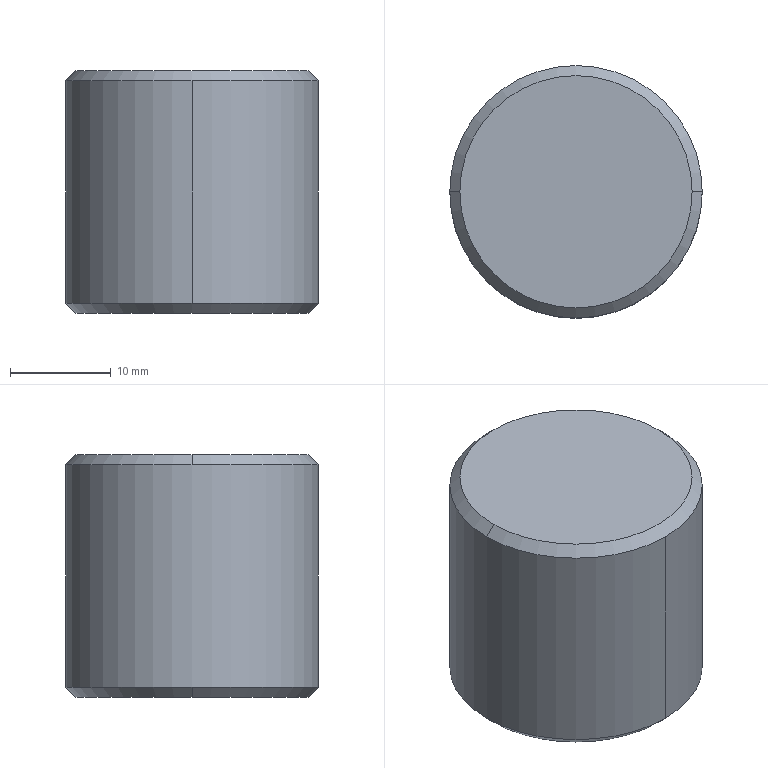Part | Creo | 1 solid | 8 faces | box 25 x 25 x 24 mm | volume 11705 mm3 | cone 4 | plane 2 | cylinder 2 | commonest cylinder face diameters 25 x2
STEP:
#1=CARTESIAN_POINT('',(-132.,-250.505,-316.));
#2=VERTEX_POINT('',#1);
#3=CARTESIAN_POINT('',(-120.5,-262.005,-316.));
#4=VERTEX_POINT('',#3);
#5=CARTESIAN_POINT('',(-132.,-262.005,-316.));
#6=DIRECTION('',(0.,0.,-1.));
#7=DIRECTION('',(0.,1.,0.));
#8=AXIS2_PLACEMENT_3D('',#5,#6,#7);
#9=CIRCLE('',#8,11.5);
#10=EDGE_CURVE('',#2,#4,#9,.T.);
#11=ORIENTED_EDGE('',*,*,#10,.F.);
#12=CARTESIAN_POINT('',(-143.5,-262.005,-316.));
#13=VERTEX_POINT('',#12);
#14=CARTESIAN_POINT('',(-132.,-262.005,-316.));
#15=DIRECTION('',(0.,0.,-1.));
#16=DIRECTION('',(-1.,0.,0.));
#17=AXIS2_PLACEMENT_3D('',#14,#15,#16);
#18=CIRCLE('',#17,11.5);
#19=EDGE_CURVE('',#13,#2,#18,.T.);
#20=ORIENTED_EDGE('',*,*,#19,.F.);
#21=CARTESIAN_POINT('',(-132.,-273.505,-316.));
#22=VERTEX_POINT('',#21);
#23=CARTESIAN_POINT('',(-132.,-262.005,-316.));
#24=DIRECTION('',(0.,0.,-1.));
#25=DIRECTION('',(0.,-1.,0.));
#26=AXIS2_PLACEMENT_3D('',#23,#24,#25);
#27=CIRCLE('',#26,11.5);
#28=EDGE_CURVE('',#22,#13,#27,.T.);
#29=ORIENTED_EDGE('',*,*,#28,.F.);
#30=CARTESIAN_POINT('',(-132.,-262.005,-316.));
#31=DIRECTION('',(0.,0.,-1.));
#32=DIRECTION('',(1.,0.,0.));
#33=AXIS2_PLACEMENT_3D('',#30,#31,#32);
#34=CIRCLE('',#33,11.5);
#35=EDGE_CURVE('',#4,#22,#34,.T.);
#36=ORIENTED_EDGE('',*,*,#35,.F.);
#37=EDGE_LOOP('',(#11,#20,#29,#36));
#38=FACE_OUTER_BOUND('',#37,.F.);
#39=CARTESIAN_POINT('',(-10.,7.995,-316.));
#40=DIRECTION('',(0.,0.,1.));
#41=DIRECTION('',(0.,-1.,0.));
#42=AXIS2_PLACEMENT_3D('',#39,#40,#41);
#43=PLANE('',#42);
#44=ADVANCED_FACE('',(#38),#43,.F.);
#45=ORIENTED_EDGE('',*,*,#19,.T.);
#46=ORIENTED_EDGE('',*,*,#10,.T.);
#47=CARTESIAN_POINT('',(-119.5,-262.005,-315.));
#48=VERTEX_POINT('',#47);
#49=CARTESIAN_POINT('',(-120.5,-262.005,-316.));
#50=DIRECTION('',(0.7071,0.,0.7071));
#51=VECTOR('',#50,1.414);
#52=LINE('',#49,#51);
#53=EDGE_CURVE('',#4,#48,#52,.T.);
#54=ORIENTED_EDGE('',*,*,#53,.T.);
#55=CARTESIAN_POINT('',(-132.,-249.505,-315.));
#56=VERTEX_POINT('',#55);
#57=CARTESIAN_POINT('',(-132.,-262.005,-315.));
#58=DIRECTION('',(0.,0.,-1.));
#59=DIRECTION('',(0.,1.,0.));
#60=AXIS2_PLACEMENT_3D('',#57,#58,#59);
#61=CIRCLE('',#60,12.5);
#62=EDGE_CURVE('',#56,#48,#61,.T.);
#63=ORIENTED_EDGE('',*,*,#62,.F.);
#64=CARTESIAN_POINT('',(-144.5,-262.005,-315.));
#65=VERTEX_POINT('',#64);
#66=CARTESIAN_POINT('',(-132.,-262.005,-315.));
#67=DIRECTION('',(0.,0.,-1.));
#68=DIRECTION('',(-1.,0.,0.));
#69=AXIS2_PLACEMENT_3D('',#66,#67,#68);
#70=CIRCLE('',#69,12.5);
#71=EDGE_CURVE('',#65,#56,#70,.T.);
#72=ORIENTED_EDGE('',*,*,#71,.F.);
#73=CARTESIAN_POINT('',(-143.5,-262.005,-316.));
#74=DIRECTION('',(-0.7071,0.,0.7071));
#75=VECTOR('',#74,1.414);
#76=LINE('',#73,#75);
#77=EDGE_CURVE('',#13,#65,#76,.T.);
#78=ORIENTED_EDGE('',*,*,#77,.F.);
#79=EDGE_LOOP('',(#45,#46,#54,#63,#72,#78));
#80=FACE_OUTER_BOUND('',#79,.F.);
#81=CARTESIAN_POINT('',(-132.,-262.005,-315.5));
#82=DIRECTION('',(0.,0.,1.));
#83=DIRECTION('',(-1.,0.,0.));
#84=AXIS2_PLACEMENT_3D('',#81,#82,#83);
#85=CONICAL_SURFACE('',#84,12.,45.);
#86=ADVANCED_FACE('',(#80),#85,.T.);
#87=ORIENTED_EDGE('',*,*,#28,.T.);
#88=ORIENTED_EDGE('',*,*,#77,.T.);
#89=CARTESIAN_POINT('',(-132.,-274.505,-315.));
#90=VERTEX_POINT('',#89);
#91=CARTESIAN_POINT('',(-132.,-262.005,-315.));
#92=DIRECTION('',(0.,0.,-1.));
#93=DIRECTION('',(0.,-1.,0.));
#94=AXIS2_PLACEMENT_3D('',#91,#92,#93);
#95=CIRCLE('',#94,12.5);
#96=EDGE_CURVE('',#90,#65,#95,.T.);
#97=ORIENTED_EDGE('',*,*,#96,.F.);
#98=CARTESIAN_POINT('',(-132.,-262.005,-315.));
#99=DIRECTION('',(0.,0.,-1.));
#100=DIRECTION('',(1.,0.,0.));
#101=AXIS2_PLACEMENT_3D('',#98,#99,#100);
#102=CIRCLE('',#101,12.5);
#103=EDGE_CURVE('',#48,#90,#102,.T.);
#104=ORIENTED_EDGE('',*,*,#103,.F.);
#105=ORIENTED_EDGE('',*,*,#53,.F.);
#106=ORIENTED_EDGE('',*,*,#35,.T.);
#107=EDGE_LOOP('',(#87,#88,#97,#104,#105,#106));
#108=FACE_OUTER_BOUND('',#107,.F.);
#109=CARTESIAN_POINT('',(-132.,-262.005,-315.5));
#110=DIRECTION('',(0.,0.,1.));
#111=DIRECTION('',(-1.,0.,0.));
#112=AXIS2_PLACEMENT_3D('',#109,#110,#111);
#113=CONICAL_SURFACE('',#112,12.,45.);
#114=ADVANCED_FACE('',(#108),#113,.T.);
#115=ORIENTED_EDGE('',*,*,#71,.T.);
#116=CARTESIAN_POINT('',(-132.,-249.505,-293.));
#117=VERTEX_POINT('',#116);
#118=CARTESIAN_POINT('',(-132.,-249.505,-315.));
#119=DIRECTION('',(0.,0.,1.));
#120=VECTOR('',#119,22.);
#121=LINE('',#118,#120);
#122=EDGE_CURVE('',#56,#117,#121,.T.);
#123=ORIENTED_EDGE('',*,*,#122,.T.);
#124=CARTESIAN_POINT('',(-144.5,-262.005,-293.));
#125=VERTEX_POINT('',#124);
#126=CARTESIAN_POINT('',(-132.,-262.005,-293.));
#127=DIRECTION('',(0.,0.,1.));
#128=DIRECTION('',(0.,1.,0.));
#129=AXIS2_PLACEMENT_3D('',#126,#127,#128);
#130=CIRCLE('',#129,12.5);
#131=EDGE_CURVE('',#117,#125,#130,.T.);
#132=ORIENTED_EDGE('',*,*,#131,.T.);
#133=CARTESIAN_POINT('',(-132.,-274.505,-293.));
#134=VERTEX_POINT('',#133);
#135=CARTESIAN_POINT('',(-132.,-262.005,-293.));
#136=DIRECTION('',(0.,0.,1.));
#137=DIRECTION('',(-1.,0.,0.));
#138=AXIS2_PLACEMENT_3D('',#135,#136,#137);
#139=CIRCLE('',#138,12.5);
#140=EDGE_CURVE('',#125,#134,#139,.T.);
#141=ORIENTED_EDGE('',*,*,#140,.T.);
#142=CARTESIAN_POINT('',(-132.,-274.505,-315.));
#143=DIRECTION('',(0.,0.,1.));
#144=VECTOR('',#143,22.);
#145=LINE('',#142,#144);
#146=EDGE_CURVE('',#90,#134,#145,.T.);
#147=ORIENTED_EDGE('',*,*,#146,.F.);
#148=ORIENTED_EDGE('',*,*,#96,.T.);
#149=EDGE_LOOP('',(#115,#123,#132,#141,#147,#148));
#150=FACE_OUTER_BOUND('',#149,.F.);
#151=CARTESIAN_POINT('',(-132.,-262.005,-316.));
#152=DIRECTION('',(0.,0.,1.));
#153=DIRECTION('',(0.,-1.,0.));
#154=AXIS2_PLACEMENT_3D('',#151,#152,#153);
#155=CYLINDRICAL_SURFACE('',#154,12.5);
#156=ADVANCED_FACE('',(#150),#155,.T.);
#157=ORIENTED_EDGE('',*,*,#103,.T.);
#158=ORIENTED_EDGE('',*,*,#146,.T.);
#159=CARTESIAN_POINT('',(-119.5,-262.005,-293.));
#160=VERTEX_POINT('',#159);
#161=CARTESIAN_POINT('',(-132.,-262.005,-293.));
#162=DIRECTION('',(0.,0.,1.));
#163=DIRECTION('',(0.,-1.,0.));
#164=AXIS2_PLACEMENT_3D('',#161,#162,#163);
#165=CIRCLE('',#164,12.5);
#166=EDGE_CURVE('',#134,#160,#165,.T.);
#167=ORIENTED_EDGE('',*,*,#166,.T.);
#168=CARTESIAN_POINT('',(-132.,-262.005,-293.));
#169=DIRECTION('',(0.,0.,1.));
#170=DIRECTION('',(1.,0.,0.));
#171=AXIS2_PLACEMENT_3D('',#168,#169,#170);
#172=CIRCLE('',#171,12.5);
#173=EDGE_CURVE('',#160,#117,#172,.T.);
#174=ORIENTED_EDGE('',*,*,#173,.T.);
#175=ORIENTED_EDGE('',*,*,#122,.F.);
#176=ORIENTED_EDGE('',*,*,#62,.T.);
#177=EDGE_LOOP('',(#157,#158,#167,#174,#175,#176));
#178=FACE_OUTER_BOUND('',#177,.F.);
#179=CARTESIAN_POINT('',(-132.,-262.005,-316.));
#180=DIRECTION('',(0.,0.,1.));
#181=DIRECTION('',(0.,-1.,0.));
#182=AXIS2_PLACEMENT_3D('',#179,#180,#181);
#183=CYLINDRICAL_SURFACE('',#182,12.5);
#184=ADVANCED_FACE('',(#178),#183,.T.);
#185=ORIENTED_EDGE('',*,*,#166,.F.);
#186=ORIENTED_EDGE('',*,*,#140,.F.);
#187=CARTESIAN_POINT('',(-143.5,-262.005,-292.));
#188=VERTEX_POINT('',#187);
#189=CARTESIAN_POINT('',(-143.5,-262.005,-292.));
#190=DIRECTION('',(-0.7071,0.,-0.7071));
#191=VECTOR('',#190,1.414);
#192=LINE('',#189,#191);
#193=EDGE_CURVE('',#188,#125,#192,.T.);
#194=ORIENTED_EDGE('',*,*,#193,.F.);
#195=CARTESIAN_POINT('',(-132.,-273.505,-292.));
#196=VERTEX_POINT('',#195);
#197=CARTESIAN_POINT('',(-132.,-262.005,-292.));
#198=DIRECTION('',(0.,0.,1.));
#199=DIRECTION('',(-1.,0.,0.));
#200=AXIS2_PLACEMENT_3D('',#197,#198,#199);
#201=CIRCLE('',#200,11.5);
#202=EDGE_CURVE('',#188,#196,#201,.T.);
#203=ORIENTED_EDGE('',*,*,#202,.T.);
#204=CARTESIAN_POINT('',(-120.5,-262.005,-292.));
#205=VERTEX_POINT('',#204);
#206=CARTESIAN_POINT('',(-132.,-262.005,-292.));
#207=DIRECTION('',(0.,0.,1.));
#208=DIRECTION('',(0.,-1.,0.));
#209=AXIS2_PLACEMENT_3D('',#206,#207,#208);
#210=CIRCLE('',#209,11.5);
#211=EDGE_CURVE('',#196,#205,#210,.T.);
#212=ORIENTED_EDGE('',*,*,#211,.T.);
#213=CARTESIAN_POINT('',(-120.5,-262.005,-292.));
#214=DIRECTION('',(0.7071,0.,-0.7071));
#215=VECTOR('',#214,1.414);
#216=LINE('',#213,#215);
#217=EDGE_CURVE('',#205,#160,#216,.T.);
#218=ORIENTED_EDGE('',*,*,#217,.T.);
#219=EDGE_LOOP('',(#185,#186,#194,#203,#212,#218));
#220=FACE_OUTER_BOUND('',#219,.F.);
#221=CARTESIAN_POINT('',(-132.,-262.005,-292.5));
#222=DIRECTION('',(0.,0.,-1.));
#223=DIRECTION('',(-1.,0.,0.));
#224=AXIS2_PLACEMENT_3D('',#221,#222,#223);
#225=CONICAL_SURFACE('',#224,12.,45.);
#226=ADVANCED_FACE('',(#220),#225,.T.);
#227=ORIENTED_EDGE('',*,*,#173,.F.);
#228=ORIENTED_EDGE('',*,*,#217,.F.);
#229=CARTESIAN_POINT('',(-132.,-250.505,-292.));
#230=VERTEX_POINT('',#229);
#231=CARTESIAN_POINT('',(-132.,-262.005,-292.));
#232=DIRECTION('',(0.,0.,1.));
#233=DIRECTION('',(1.,0.,0.));
#234=AXIS2_PLACEMENT_3D('',#231,#232,#233);
#235=CIRCLE('',#234,11.5);
#236=EDGE_CURVE('',#205,#230,#235,.T.);
#237=ORIENTED_EDGE('',*,*,#236,.T.);
#238=CARTESIAN_POINT('',(-132.,-262.005,-292.));
#239=DIRECTION('',(0.,0.,1.));
#240=DIRECTION('',(0.,1.,0.));
#241=AXIS2_PLACEMENT_3D('',#238,#239,#240);
#242=CIRCLE('',#241,11.5);
#243=EDGE_CURVE('',#230,#188,#242,.T.);
#244=ORIENTED_EDGE('',*,*,#243,.T.);
#245=ORIENTED_EDGE('',*,*,#193,.T.);
#246=ORIENTED_EDGE('',*,*,#131,.F.);
#247=EDGE_LOOP('',(#227,#228,#237,#244,#245,#246));
#248=FACE_OUTER_BOUND('',#247,.F.);
#249=CARTESIAN_POINT('',(-132.,-262.005,-292.5));
#250=DIRECTION('',(0.,0.,-1.));
#251=DIRECTION('',(-1.,0.,0.));
#252=AXIS2_PLACEMENT_3D('',#249,#250,#251);
#253=CONICAL_SURFACE('',#252,12.,45.);
#254=ADVANCED_FACE('',(#248),#253,.T.);
#255=ORIENTED_EDGE('',*,*,#211,.F.);
#256=ORIENTED_EDGE('',*,*,#202,.F.);
#257=ORIENTED_EDGE('',*,*,#243,.F.);
#258=ORIENTED_EDGE('',*,*,#236,.F.);
#259=EDGE_LOOP('',(#255,#256,#257,#258));
#260=FACE_OUTER_BOUND('',#259,.F.);
#261=CARTESIAN_POINT('',(-10.,7.995,-292.));
#262=DIRECTION('',(0.,0.,1.));
#263=DIRECTION('',(0.,-1.,0.));
#264=AXIS2_PLACEMENT_3D('',#261,#262,#263);
#265=PLANE('',#264);
#266=ADVANCED_FACE('',(#260),#265,.T.);
#267=CLOSED_SHELL('',(#44,#86,#114,#156,#184,#226,#254,#266));
#268=MANIFOLD_SOLID_BREP('',#267);
#269=(LENGTH_UNIT()NAMED_UNIT(*)SI_UNIT(.MILLI.,.METRE.));
#270=UNCERTAINTY_MEASURE_WITH_UNIT(LENGTH_MEASURE(0.004273),#269,'','');
#271=(NAMED_UNIT(*)PLANE_ANGLE_UNIT()SI_UNIT($,.RADIAN.));
#272=PLANE_ANGLE_MEASURE_WITH_UNIT(PLANE_ANGLE_MEASURE(0.01745),#271);
#273=(CONVERSION_BASED_UNIT('DEGREE',#272)NAMED_UNIT(*)PLANE_ANGLE_UNIT());
#274=(NAMED_UNIT(*)SI_UNIT($,.STERADIAN.)SOLID_ANGLE_UNIT());
#275=(GEOMETRIC_REPRESENTATION_CONTEXT(3)GLOBAL_UNCERTAINTY_ASSIGNED_CONTEXT((#270))GLOBAL_UNIT_ASSIGNED_CONTEXT((#269,#273,#274))REPRESENTATION_CONTEXT('',''));
#276=ADVANCED_BREP_SHAPE_REPRESENTATION('',(#268),#275);